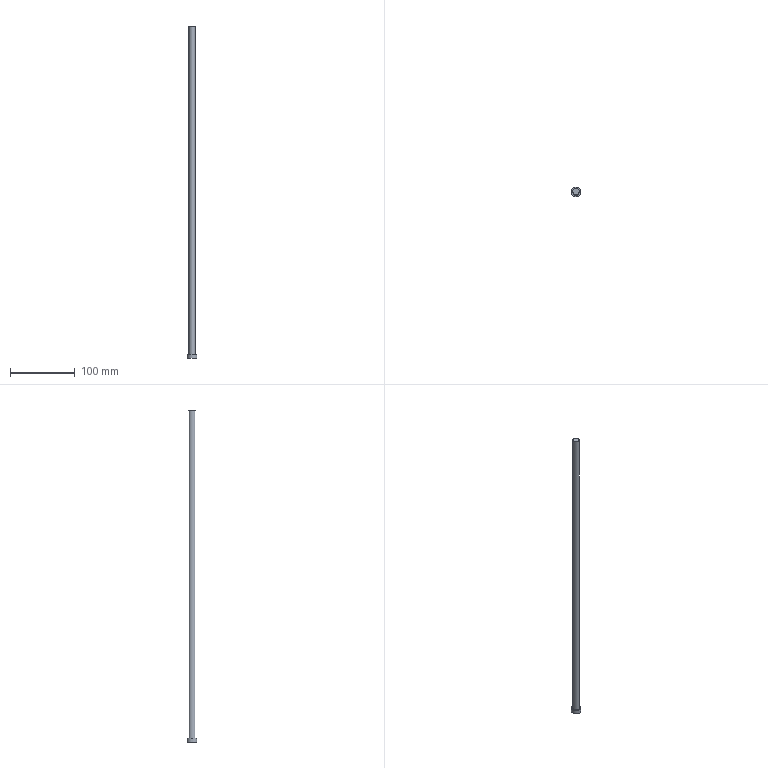Part | STEP file | solid 71 | 1 solid | 5 faces | box 15 x 15 x 512.106 mm | volume 40810 mm3 | plane 3 | cylinder 2 | commonest cylinder face diameters 10 x1 15 x1